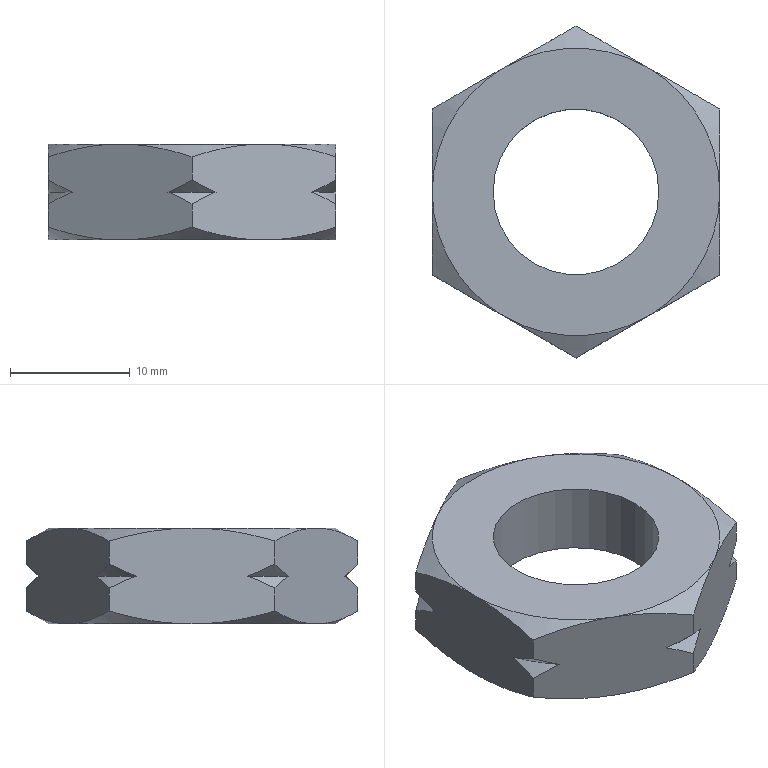Part | STEP file | HXGR200008-06-03-04_M16 | 1 solid | 39 faces | box 24 x 27.713 x 8 mm | volume 2454 mm3 | cone 26 | plane 9 | cylinder 4 | commonest cylinder face diameters 13.835 x2 19.5 x2
STEP:
#1=CARTESIAN_POINT('',(9.75,0.,2.));
#2=VERTEX_POINT('',#1);
#3=CARTESIAN_POINT('',(-9.75,0.,2.));
#4=VERTEX_POINT('',#3);
#5=CARTESIAN_POINT('',(0.,0.,2.));
#6=DIRECTION('',(0.,0.,-1.));
#7=DIRECTION('',(-1.,0.,0.));
#8=AXIS2_PLACEMENT_3D('',#5,#6,#7);
#9=CIRCLE('',#8,9.75);
#10=EDGE_CURVE('',#2,#4,#9,.T.);
#11=ORIENTED_EDGE('',*,*,#10,.F.);
#12=CARTESIAN_POINT('',(9.75,0.,0.));
#13=VERTEX_POINT('',#12);
#14=CARTESIAN_POINT('',(9.75,0.,2.));
#15=DIRECTION('',(0.,0.,-1.));
#16=VECTOR('',#15,1000.);
#17=LINE('',#14,#16);
#18=EDGE_CURVE('',#2,#13,#17,.T.);
#19=ORIENTED_EDGE('',*,*,#18,.T.);
#20=CARTESIAN_POINT('',(-9.75,0.,0.));
#21=VERTEX_POINT('',#20);
#22=CARTESIAN_POINT('',(0.,0.,0.));
#23=DIRECTION('',(0.,0.,-1.));
#24=DIRECTION('',(-1.,0.,0.));
#25=AXIS2_PLACEMENT_3D('',#22,#23,#24);
#26=CIRCLE('',#25,9.75);
#27=EDGE_CURVE('',#13,#21,#26,.T.);
#28=ORIENTED_EDGE('',*,*,#27,.T.);
#29=CARTESIAN_POINT('',(-9.75,0.,2.));
#30=DIRECTION('',(0.,0.,-1.));
#31=VECTOR('',#30,1000.);
#32=LINE('',#29,#31);
#33=EDGE_CURVE('',#4,#21,#32,.T.);
#34=ORIENTED_EDGE('',*,*,#33,.F.);
#35=EDGE_LOOP('',(#11,#19,#28,#34));
#36=FACE_OUTER_BOUND('',#35,.T.);
#37=CARTESIAN_POINT('',(0.,0.,2.));
#38=DIRECTION('',(0.,0.,-1.));
#39=DIRECTION('',(-1.,0.,0.));
#40=AXIS2_PLACEMENT_3D('',#37,#38,#39);
#41=CYLINDRICAL_SURFACE('',#40,9.75);
#42=ADVANCED_FACE('',(#36),#41,.F.);
#43=CARTESIAN_POINT('',(-6.918,0.,8.));
#44=VERTEX_POINT('',#43);
#45=CARTESIAN_POINT('',(6.918,0.,8.));
#46=VERTEX_POINT('',#45);
#47=CARTESIAN_POINT('',(0.,0.,8.));
#48=DIRECTION('',(0.,0.,1.));
#49=DIRECTION('',(1.,0.,0.));
#50=AXIS2_PLACEMENT_3D('',#47,#48,#49);
#51=CIRCLE('',#50,6.918);
#52=EDGE_CURVE('',#44,#46,#51,.T.);
#53=ORIENTED_EDGE('',*,*,#52,.T.);
#54=CARTESIAN_POINT('',(6.918,0.,2.));
#55=VERTEX_POINT('',#54);
#56=CARTESIAN_POINT('',(6.918,0.,8.));
#57=DIRECTION('',(0.,0.,-1.));
#58=VECTOR('',#57,1000.);
#59=LINE('',#56,#58);
#60=EDGE_CURVE('',#46,#55,#59,.T.);
#61=ORIENTED_EDGE('',*,*,#60,.T.);
#62=CARTESIAN_POINT('',(-6.918,0.,2.));
#63=VERTEX_POINT('',#62);
#64=CARTESIAN_POINT('',(0.,0.,2.));
#65=DIRECTION('',(0.,0.,-1.));
#66=DIRECTION('',(-1.,0.,0.));
#67=AXIS2_PLACEMENT_3D('',#64,#65,#66);
#68=CIRCLE('',#67,6.918);
#69=EDGE_CURVE('',#55,#63,#68,.T.);
#70=ORIENTED_EDGE('',*,*,#69,.T.);
#71=CARTESIAN_POINT('',(-6.918,0.,8.));
#72=DIRECTION('',(0.,0.,-1.));
#73=VECTOR('',#72,1000.);
#74=LINE('',#71,#73);
#75=EDGE_CURVE('',#44,#63,#74,.T.);
#76=ORIENTED_EDGE('',*,*,#75,.F.);
#77=EDGE_LOOP('',(#53,#61,#70,#76));
#78=FACE_OUTER_BOUND('',#77,.T.);
#79=CARTESIAN_POINT('',(0.,0.,8.));
#80=DIRECTION('',(0.,0.,-1.));
#81=DIRECTION('',(-1.,0.,0.));
#82=AXIS2_PLACEMENT_3D('',#79,#80,#81);
#83=CYLINDRICAL_SURFACE('',#82,6.918);
#84=ADVANCED_FACE('',(#78),#83,.F.);
#85=CARTESIAN_POINT('',(9.996,8.085,4.));
#86=VERTEX_POINT('',#85);
#87=CARTESIAN_POINT('',(12.,6.928,5.));
#88=VERTEX_POINT('',#87);
#89=CARTESIAN_POINT('',(9.996,8.085,4.));
#90=CARTESIAN_POINT('',(10.339,7.887,4.142));
#91=CARTESIAN_POINT('',(10.68,7.69,4.3));
#92=CARTESIAN_POINT('',(11.348,7.305,4.635));
#93=CARTESIAN_POINT('',(11.676,7.115,4.813));
#94=CARTESIAN_POINT('',(12.,6.928,5.));
#95=B_SPLINE_CURVE_WITH_KNOTS('',3,(#89,#90,#91,#92,#93,#94),.UNSPECIFIED.,.F.,.F.,(4,2,4),(0.02361,0.02487,0.02612),.UNSPECIFIED.);
#96=EDGE_CURVE('',#86,#88,#95,.T.);
#97=ORIENTED_EDGE('',*,*,#96,.F.);
#98=CARTESIAN_POINT('',(12.,6.928,3.));
#99=VERTEX_POINT('',#98);
#100=CARTESIAN_POINT('',(12.,6.928,3.));
#101=CARTESIAN_POINT('',(11.348,7.305,3.377));
#102=CARTESIAN_POINT('',(10.682,7.689,3.716));
#103=CARTESIAN_POINT('',(9.996,8.085,4.));
#104=B_SPLINE_CURVE_WITH_KNOTS('',3,(#100,#101,#102,#103),.UNSPECIFIED.,.F.,.F.,(4,4),(0.01167,0.01419),.UNSPECIFIED.);
#105=EDGE_CURVE('',#99,#86,#104,.T.);
#106=ORIENTED_EDGE('',*,*,#105,.F.);
#107=CARTESIAN_POINT('',(12.,6.928,1.072));
#108=VERTEX_POINT('',#107);
#109=CARTESIAN_POINT('',(12.,6.928,8.));
#110=DIRECTION('',(0.,0.,-1.));
#111=VECTOR('',#110,1000.);
#112=LINE('',#109,#111);
#113=EDGE_CURVE('',#99,#108,#112,.T.);
#114=ORIENTED_EDGE('',*,*,#113,.T.);
#115=CARTESIAN_POINT('',(6.,10.392,0.));
#116=VERTEX_POINT('',#115);
#117=CARTESIAN_POINT('',(6.,10.392,0.));
#118=CARTESIAN_POINT('',(6.509,10.098,0.));
#119=CARTESIAN_POINT('',(7.021,9.803,0.02533));
#120=CARTESIAN_POINT('',(8.033,9.219,0.1234));
#121=CARTESIAN_POINT('',(8.535,8.929,0.196));
#122=CARTESIAN_POINT('',(10.034,8.063,0.476));
#123=CARTESIAN_POINT('',(11.021,7.493,0.7454));
#124=CARTESIAN_POINT('',(12.,6.928,1.072));
#125=B_SPLINE_CURVE_WITH_KNOTS('',3,(#117,#118,#119,#120,#121,#122,#123,#124),.UNSPECIFIED.,.F.,.F.,(4,2,2,4),(0.00701,0.008756,0.0105,0.01399),.UNSPECIFIED.);
#126=EDGE_CURVE('',#116,#108,#125,.T.);
#127=ORIENTED_EDGE('',*,*,#126,.F.);
#128=CARTESIAN_POINT('',(0.,13.856,1.072));
#129=VERTEX_POINT('',#128);
#130=CARTESIAN_POINT('',(0.,13.856,1.072));
#131=CARTESIAN_POINT('',(0.9815,13.29,0.7446));
#132=CARTESIAN_POINT('',(1.97,12.719,0.4751));
#133=CARTESIAN_POINT('',(3.968,11.565,0.1021));
#134=CARTESIAN_POINT('',(4.978,10.982,0.));
#135=CARTESIAN_POINT('',(6.,10.392,0.));
#136=B_SPLINE_CURVE_WITH_KNOTS('',3,(#130,#131,#132,#133,#134,#135),.UNSPECIFIED.,.F.,.F.,(4,2,4),(0.000000238,0.003505,0.00701),.UNSPECIFIED.);
#137=EDGE_CURVE('',#129,#116,#136,.T.);
#138=ORIENTED_EDGE('',*,*,#137,.F.);
#139=CARTESIAN_POINT('',(0.,13.856,3.));
#140=VERTEX_POINT('',#139);
#141=CARTESIAN_POINT('',(0.,13.856,8.));
#142=DIRECTION('',(0.,0.,-1.));
#143=VECTOR('',#142,1000.);
#144=LINE('',#141,#143);
#145=EDGE_CURVE('',#140,#129,#144,.T.);
#146=ORIENTED_EDGE('',*,*,#145,.F.);
#147=CARTESIAN_POINT('',(2.004,12.699,4.));
#148=VERTEX_POINT('',#147);
#149=CARTESIAN_POINT('',(2.004,12.699,4.));
#150=CARTESIAN_POINT('',(1.661,12.898,3.858));
#151=CARTESIAN_POINT('',(1.32,13.094,3.7));
#152=CARTESIAN_POINT('',(0.6518,13.48,3.365));
#153=CARTESIAN_POINT('',(0.3236,13.67,3.187));
#154=CARTESIAN_POINT('',(0.,13.856,3.));
#155=B_SPLINE_CURVE_WITH_KNOTS('',3,(#149,#150,#151,#152,#153,#154),.UNSPECIFIED.,.F.,.F.,(4,2,4),(0.02361,0.02487,0.02612),.UNSPECIFIED.);
#156=EDGE_CURVE('',#148,#140,#155,.T.);
#157=ORIENTED_EDGE('',*,*,#156,.F.);
#158=CARTESIAN_POINT('',(0.,13.856,5.));
#159=VERTEX_POINT('',#158);
#160=CARTESIAN_POINT('',(0.,13.856,5.));
#161=CARTESIAN_POINT('',(0.6523,13.48,4.623));
#162=CARTESIAN_POINT('',(1.318,13.095,4.284));
#163=CARTESIAN_POINT('',(2.004,12.699,4.));
#164=B_SPLINE_CURVE_WITH_KNOTS('',3,(#160,#161,#162,#163),.UNSPECIFIED.,.F.,.F.,(4,4),(0.01167,0.01419),.UNSPECIFIED.);
#165=EDGE_CURVE('',#159,#148,#164,.T.);
#166=ORIENTED_EDGE('',*,*,#165,.F.);
#167=CARTESIAN_POINT('',(0.,13.856,6.928));
#168=VERTEX_POINT('',#167);
#169=CARTESIAN_POINT('',(0.,13.856,8.));
#170=DIRECTION('',(0.,0.,-1.));
#171=VECTOR('',#170,1000.);
#172=LINE('',#169,#171);
#173=EDGE_CURVE('',#168,#159,#172,.T.);
#174=ORIENTED_EDGE('',*,*,#173,.F.);
#175=CARTESIAN_POINT('',(6.,10.392,8.));
#176=VERTEX_POINT('',#175);
#177=CARTESIAN_POINT('',(6.,10.392,8.));
#178=CARTESIAN_POINT('',(5.491,10.686,8.));
#179=CARTESIAN_POINT('',(4.979,10.982,7.975));
#180=CARTESIAN_POINT('',(3.967,11.566,7.877));
#181=CARTESIAN_POINT('',(3.465,11.856,7.804));
#182=CARTESIAN_POINT('',(1.966,12.721,7.524));
#183=CARTESIAN_POINT('',(0.9791,13.291,7.255));
#184=CARTESIAN_POINT('',(0.,13.856,6.928));
#185=B_SPLINE_CURVE_WITH_KNOTS('',3,(#177,#178,#179,#180,#181,#182,#183,#184),.UNSPECIFIED.,.F.,.F.,(4,2,2,4),(0.00701,0.008756,0.0105,0.01399),.UNSPECIFIED.);
#186=EDGE_CURVE('',#176,#168,#185,.T.);
#187=ORIENTED_EDGE('',*,*,#186,.F.);
#188=CARTESIAN_POINT('',(12.,6.928,6.928));
#189=VERTEX_POINT('',#188);
#190=CARTESIAN_POINT('',(12.,6.928,6.928));
#191=CARTESIAN_POINT('',(11.018,7.495,7.255));
#192=CARTESIAN_POINT('',(10.03,8.066,7.525));
#193=CARTESIAN_POINT('',(8.032,9.219,7.898));
#194=CARTESIAN_POINT('',(7.022,9.802,8.));
#195=CARTESIAN_POINT('',(6.,10.392,8.));
#196=B_SPLINE_CURVE_WITH_KNOTS('',3,(#190,#191,#192,#193,#194,#195),.UNSPECIFIED.,.F.,.F.,(4,2,4),(0.000000238,0.003505,0.00701),.UNSPECIFIED.);
#197=EDGE_CURVE('',#189,#176,#196,.T.);
#198=ORIENTED_EDGE('',*,*,#197,.F.);
#199=CARTESIAN_POINT('',(12.,6.928,8.));
#200=DIRECTION('',(0.,0.,-1.));
#201=VECTOR('',#200,1000.);
#202=LINE('',#199,#201);
#203=EDGE_CURVE('',#189,#88,#202,.T.);
#204=ORIENTED_EDGE('',*,*,#203,.T.);
#205=EDGE_LOOP('',(#97,#106,#114,#127,#138,#146,#157,#166,#174,#187,#198,#204));
#206=FACE_OUTER_BOUND('',#205,.T.);
#207=CARTESIAN_POINT('',(12.,6.928,8.));
#208=DIRECTION('',(-0.5,-0.866,0.));
#209=DIRECTION('',(0.866,-0.5,0.));
#210=AXIS2_PLACEMENT_3D('',#207,#208,#209);
#211=PLANE('',#210);
#212=ADVANCED_FACE('',(#206),#211,.F.);
#213=CARTESIAN_POINT('',(-2.004,12.699,4.));
#214=VERTEX_POINT('',#213);
#215=CARTESIAN_POINT('',(-2.004,12.699,4.));
#216=CARTESIAN_POINT('',(-1.661,12.898,4.142));
#217=CARTESIAN_POINT('',(-1.32,13.094,4.3));
#218=CARTESIAN_POINT('',(-0.6518,13.48,4.635));
#219=CARTESIAN_POINT('',(-0.3236,13.67,4.813));
#220=CARTESIAN_POINT('',(0.,13.856,5.));
#221=B_SPLINE_CURVE_WITH_KNOTS('',3,(#215,#216,#217,#218,#219,#220),.UNSPECIFIED.,.F.,.F.,(4,2,4),(0.02361,0.02487,0.02612),.UNSPECIFIED.);
#222=EDGE_CURVE('',#214,#159,#221,.T.);
#223=ORIENTED_EDGE('',*,*,#222,.F.);
#224=CARTESIAN_POINT('',(0.,13.856,3.));
#225=CARTESIAN_POINT('',(-0.6523,13.48,3.377));
#226=CARTESIAN_POINT('',(-1.318,13.095,3.716));
#227=CARTESIAN_POINT('',(-2.004,12.699,4.));
#228=B_SPLINE_CURVE_WITH_KNOTS('',3,(#224,#225,#226,#227),.UNSPECIFIED.,.F.,.F.,(4,4),(0.01167,0.01419),.UNSPECIFIED.);
#229=EDGE_CURVE('',#140,#214,#228,.T.);
#230=ORIENTED_EDGE('',*,*,#229,.F.);
#231=ORIENTED_EDGE('',*,*,#145,.T.);
#232=CARTESIAN_POINT('',(-6.,10.392,0.));
#233=VERTEX_POINT('',#232);
#234=CARTESIAN_POINT('',(-6.,10.392,0.));
#235=CARTESIAN_POINT('',(-5.491,10.686,0.));
#236=CARTESIAN_POINT('',(-4.979,10.982,0.02533));
#237=CARTESIAN_POINT('',(-3.967,11.566,0.1234));
#238=CARTESIAN_POINT('',(-3.465,11.856,0.196));
#239=CARTESIAN_POINT('',(-1.966,12.721,0.476));
#240=CARTESIAN_POINT('',(-0.9791,13.291,0.7454));
#241=CARTESIAN_POINT('',(0.,13.856,1.072));
#242=B_SPLINE_CURVE_WITH_KNOTS('',3,(#234,#235,#236,#237,#238,#239,#240,#241),.UNSPECIFIED.,.F.,.F.,(4,2,2,4),(0.00701,0.008756,0.0105,0.01399),.UNSPECIFIED.);
#243=EDGE_CURVE('',#233,#129,#242,.T.);
#244=ORIENTED_EDGE('',*,*,#243,.F.);
#245=CARTESIAN_POINT('',(-12.,6.928,1.072));
#246=VERTEX_POINT('',#245);
#247=CARTESIAN_POINT('',(-12.,6.928,1.072));
#248=CARTESIAN_POINT('',(-11.018,7.495,0.7446));
#249=CARTESIAN_POINT('',(-10.03,8.066,0.4751));
#250=CARTESIAN_POINT('',(-8.032,9.219,0.1021));
#251=CARTESIAN_POINT('',(-7.022,9.802,0.));
#252=CARTESIAN_POINT('',(-6.,10.392,0.));
#253=B_SPLINE_CURVE_WITH_KNOTS('',3,(#247,#248,#249,#250,#251,#252),.UNSPECIFIED.,.F.,.F.,(4,2,4),(0.000000238,0.003505,0.00701),.UNSPECIFIED.);
#254=EDGE_CURVE('',#246,#233,#253,.T.);
#255=ORIENTED_EDGE('',*,*,#254,.F.);
#256=CARTESIAN_POINT('',(-12.,6.928,3.));
#257=VERTEX_POINT('',#256);
#258=CARTESIAN_POINT('',(-12.,6.928,8.));
#259=DIRECTION('',(0.,0.,-1.));
#260=VECTOR('',#259,1000.);
#261=LINE('',#258,#260);
#262=EDGE_CURVE('',#257,#246,#261,.T.);
#263=ORIENTED_EDGE('',*,*,#262,.F.);
#264=CARTESIAN_POINT('',(-9.996,8.085,4.));
#265=VERTEX_POINT('',#264);
#266=CARTESIAN_POINT('',(-9.996,8.085,4.));
#267=CARTESIAN_POINT('',(-10.339,7.887,3.858));
#268=CARTESIAN_POINT('',(-10.68,7.69,3.7));
#269=CARTESIAN_POINT('',(-11.348,7.305,3.365));
#270=CARTESIAN_POINT('',(-11.676,7.115,3.187));
#271=CARTESIAN_POINT('',(-12.,6.928,3.));
#272=B_SPLINE_CURVE_WITH_KNOTS('',3,(#266,#267,#268,#269,#270,#271),.UNSPECIFIED.,.F.,.F.,(4,2,4),(0.02361,0.02487,0.02612),.UNSPECIFIED.);
#273=EDGE_CURVE('',#265,#257,#272,.T.);
#274=ORIENTED_EDGE('',*,*,#273,.F.);
#275=CARTESIAN_POINT('',(-12.,6.928,5.));
#276=VERTEX_POINT('',#275);
#277=CARTESIAN_POINT('',(-12.,6.928,5.));
#278=CARTESIAN_POINT('',(-11.348,7.305,4.623));
#279=CARTESIAN_POINT('',(-10.682,7.689,4.284));
#280=CARTESIAN_POINT('',(-9.996,8.085,4.));
#281=B_SPLINE_CURVE_WITH_KNOTS('',3,(#277,#278,#279,#280),.UNSPECIFIED.,.F.,.F.,(4,4),(0.01167,0.01419),.UNSPECIFIED.);
#282=EDGE_CURVE('',#276,#265,#281,.T.);
#283=ORIENTED_EDGE('',*,*,#282,.F.);
#284=CARTESIAN_POINT('',(-12.,6.928,6.928));
#285=VERTEX_POINT('',#284);
#286=CARTESIAN_POINT('',(-12.,6.928,8.));
#287=DIRECTION('',(0.,0.,-1.));
#288=VECTOR('',#287,1000.);
#289=LINE('',#286,#288);
#290=EDGE_CURVE('',#285,#276,#289,.T.);
#291=ORIENTED_EDGE('',*,*,#290,.F.);
#292=CARTESIAN_POINT('',(-6.,10.392,8.));
#293=VERTEX_POINT('',#292);
#294=CARTESIAN_POINT('',(-6.,10.392,8.));
#295=CARTESIAN_POINT('',(-6.509,10.098,8.));
#296=CARTESIAN_POINT('',(-7.021,9.803,7.975));
#297=CARTESIAN_POINT('',(-8.033,9.219,7.877));
#298=CARTESIAN_POINT('',(-8.535,8.929,7.804));
#299=CARTESIAN_POINT('',(-10.034,8.063,7.524));
#300=CARTESIAN_POINT('',(-11.021,7.493,7.255));
#301=CARTESIAN_POINT('',(-12.,6.928,6.928));
#302=B_SPLINE_CURVE_WITH_KNOTS('',3,(#294,#295,#296,#297,#298,#299,#300,#301),.UNSPECIFIED.,.F.,.F.,(4,2,2,4),(0.00701,0.008756,0.0105,0.01399),.UNSPECIFIED.);
#303=EDGE_CURVE('',#293,#285,#302,.T.);
#304=ORIENTED_EDGE('',*,*,#303,.F.);
#305=CARTESIAN_POINT('',(0.,13.856,6.928));
#306=CARTESIAN_POINT('',(-0.9815,13.29,7.255));
#307=CARTESIAN_POINT('',(-1.97,12.719,7.525));
#308=CARTESIAN_POINT('',(-3.968,11.565,7.898));
#309=CARTESIAN_POINT('',(-4.978,10.982,8.));
#310=CARTESIAN_POINT('',(-6.,10.392,8.));
#311=B_SPLINE_CURVE_WITH_KNOTS('',3,(#305,#306,#307,#308,#309,#310),.UNSPECIFIED.,.F.,.F.,(4,2,4),(0.000000238,0.003505,0.00701),.UNSPECIFIED.);
#312=EDGE_CURVE('',#168,#293,#311,.T.);
#313=ORIENTED_EDGE('',*,*,#312,.F.);
#314=ORIENTED_EDGE('',*,*,#173,.T.);
#315=EDGE_LOOP('',(#223,#230,#231,#244,#255,#263,#274,#283,#291,#304,#313,#314));
#316=FACE_OUTER_BOUND('',#315,.T.);
#317=CARTESIAN_POINT('',(0.,13.856,8.));
#318=DIRECTION('',(0.5,-0.866,0.));
#319=DIRECTION('',(0.866,0.5,0.));
#320=AXIS2_PLACEMENT_3D('',#317,#318,#319);
#321=PLANE('',#320);
#322=ADVANCED_FACE('',(#316),#321,.F.);
#323=CARTESIAN_POINT('',(-12.,4.614,4.));
#324=VERTEX_POINT('',#323);
#325=CARTESIAN_POINT('',(-12.,4.614,4.));
#326=CARTESIAN_POINT('',(-12.,5.408,4.285));
#327=CARTESIAN_POINT('',(-12.,6.176,4.624));
#328=CARTESIAN_POINT('',(-12.,6.928,5.));
#329=B_SPLINE_CURVE_WITH_KNOTS('',3,(#325,#326,#327,#328),.UNSPECIFIED.,.F.,.F.,(4,4),(0.02193,0.02445),.UNSPECIFIED.);
#330=EDGE_CURVE('',#324,#276,#329,.T.);
#331=ORIENTED_EDGE('',*,*,#330,.F.);
#332=CARTESIAN_POINT('',(-12.,6.928,3.));
#333=CARTESIAN_POINT('',(-12.,6.552,3.188));
#334=CARTESIAN_POINT('',(-12.,6.17,3.368));
#335=CARTESIAN_POINT('',(-12.,5.398,3.703));
#336=CARTESIAN_POINT('',(-12.,5.008,3.859));
#337=CARTESIAN_POINT('',(-12.,4.614,4.));
#338=B_SPLINE_CURVE_WITH_KNOTS('',3,(#332,#333,#334,#335,#336,#337),.UNSPECIFIED.,.F.,.F.,(4,2,4),(0.01002,0.01127,0.01252),.UNSPECIFIED.);
#339=EDGE_CURVE('',#257,#324,#338,.T.);
#340=ORIENTED_EDGE('',*,*,#339,.F.);
#341=ORIENTED_EDGE('',*,*,#262,.T.);
#342=CARTESIAN_POINT('',(-12.,0.,0.));
#343=VERTEX_POINT('',#342);
#344=CARTESIAN_POINT('',(-12.,0.,0.));
#345=CARTESIAN_POINT('',(-12.,0.5865,0.));
#346=CARTESIAN_POINT('',(-12.,1.176,0.02506));
#347=CARTESIAN_POINT('',(-12.,2.355,0.1242));
#348=CARTESIAN_POINT('',(-12.,2.939,0.1976));
#349=CARTESIAN_POINT('',(-12.,4.673,0.4791));
#350=CARTESIAN_POINT('',(-12.,5.808,0.7483));
#351=CARTESIAN_POINT('',(-12.,6.928,1.072));
#352=B_SPLINE_CURVE_WITH_KNOTS('',3,(#344,#345,#346,#347,#348,#349,#350,#351),.UNSPECIFIED.,.F.,.F.,(4,2,2,4),(0.01983,0.02158,0.02334,0.02685),.UNSPECIFIED.);
#353=EDGE_CURVE('',#343,#246,#352,.T.);
#354=ORIENTED_EDGE('',*,*,#353,.F.);
#355=CARTESIAN_POINT('',(-12.,-6.928,1.072));
#356=VERTEX_POINT('',#355);
#357=CARTESIAN_POINT('',(-12.,-6.928,1.072));
#358=CARTESIAN_POINT('',(-12.,-5.8,0.7461));
#359=CARTESIAN_POINT('',(-12.,-4.647,0.4736));
#360=CARTESIAN_POINT('',(-12.,-2.335,0.1008));
#361=CARTESIAN_POINT('',(-12.,-1.172,0.));
#362=CARTESIAN_POINT('',(-12.,0.,0.));
#363=B_SPLINE_CURVE_WITH_KNOTS('',3,(#357,#358,#359,#360,#361,#362),.UNSPECIFIED.,.F.,.F.,(4,2,4),(0.01282,0.01632,0.01983),.UNSPECIFIED.);
#364=EDGE_CURVE('',#356,#343,#363,.T.);
#365=ORIENTED_EDGE('',*,*,#364,.F.);
#366=CARTESIAN_POINT('',(-12.,-6.928,3.));
#367=VERTEX_POINT('',#366);
#368=CARTESIAN_POINT('',(-12.,-6.928,8.));
#369=DIRECTION('',(0.,0.,-1.));
#370=VECTOR('',#369,1000.);
#371=LINE('',#368,#370);
#372=EDGE_CURVE('',#367,#356,#371,.T.);
#373=ORIENTED_EDGE('',*,*,#372,.F.);
#374=CARTESIAN_POINT('',(-12.,-4.614,4.));
#375=VERTEX_POINT('',#374);
#376=CARTESIAN_POINT('',(-12.,-4.614,4.));
#377=CARTESIAN_POINT('',(-12.,-5.408,3.715));
#378=CARTESIAN_POINT('',(-12.,-6.176,3.376));
#379=CARTESIAN_POINT('',(-12.,-6.928,3.));
#380=B_SPLINE_CURVE_WITH_KNOTS('',3,(#376,#377,#378,#379),.UNSPECIFIED.,.F.,.F.,(4,4),(0.02193,0.02445),.UNSPECIFIED.);
#381=EDGE_CURVE('',#375,#367,#380,.T.);
#382=ORIENTED_EDGE('',*,*,#381,.F.);
#383=CARTESIAN_POINT('',(-12.,-6.928,5.));
#384=VERTEX_POINT('',#383);
#385=CARTESIAN_POINT('',(-12.,-6.928,5.));
#386=CARTESIAN_POINT('',(-12.,-6.552,4.812));
#387=CARTESIAN_POINT('',(-12.,-6.17,4.632));
#388=CARTESIAN_POINT('',(-12.,-5.398,4.297));
#389=CARTESIAN_POINT('',(-12.,-5.008,4.141));
#390=CARTESIAN_POINT('',(-12.,-4.614,4.));
#391=B_SPLINE_CURVE_WITH_KNOTS('',3,(#385,#386,#387,#388,#389,#390),.UNSPECIFIED.,.F.,.F.,(4,2,4),(0.01002,0.01127,0.01252),.UNSPECIFIED.);
#392=EDGE_CURVE('',#384,#375,#391,.T.);
#393=ORIENTED_EDGE('',*,*,#392,.F.);
#394=CARTESIAN_POINT('',(-12.,-6.928,6.928));
#395=VERTEX_POINT('',#394);
#396=CARTESIAN_POINT('',(-12.,-6.928,8.));
#397=DIRECTION('',(0.,0.,-1.));
#398=VECTOR('',#397,1000.);
#399=LINE('',#396,#398);
#400=EDGE_CURVE('',#395,#384,#399,.T.);
#401=ORIENTED_EDGE('',*,*,#400,.F.);
#402=CARTESIAN_POINT('',(-12.,0.,8.));
#403=VERTEX_POINT('',#402);
#404=CARTESIAN_POINT('',(-12.,0.,8.));
#405=CARTESIAN_POINT('',(-12.,-1.172,8.));
#406=CARTESIAN_POINT('',(-12.,-2.335,7.899));
#407=CARTESIAN_POINT('',(-12.,-4.647,7.526));
#408=CARTESIAN_POINT('',(-12.,-5.8,7.254));
#409=CARTESIAN_POINT('',(-12.,-6.928,6.928));
#410=B_SPLINE_CURVE_WITH_KNOTS('',3,(#404,#405,#406,#407,#408,#409),.UNSPECIFIED.,.F.,.F.,(4,2,4),(0.04318,0.04669,0.05019),.UNSPECIFIED.);
#411=EDGE_CURVE('',#403,#395,#410,.T.);
#412=ORIENTED_EDGE('',*,*,#411,.F.);
#413=CARTESIAN_POINT('',(-12.,6.928,6.928));
#414=CARTESIAN_POINT('',(-12.,5.808,7.252));
#415=CARTESIAN_POINT('',(-12.,4.673,7.521));
#416=CARTESIAN_POINT('',(-12.,2.939,7.802));
#417=CARTESIAN_POINT('',(-12.,2.355,7.876));
#418=CARTESIAN_POINT('',(-12.,1.176,7.975));
#419=CARTESIAN_POINT('',(-12.,0.5865,8.));
#420=CARTESIAN_POINT('',(-12.,0.,8.));
#421=B_SPLINE_CURVE_WITH_KNOTS('',3,(#413,#414,#415,#416,#417,#418,#419,#420),.UNSPECIFIED.,.F.,.F.,(4,2,2,4),(0.03616,0.03967,0.04143,0.04318),.UNSPECIFIED.);
#422=EDGE_CURVE('',#285,#403,#421,.T.);
#423=ORIENTED_EDGE('',*,*,#422,.F.);
#424=ORIENTED_EDGE('',*,*,#290,.T.);
#425=EDGE_LOOP('',(#331,#340,#341,#354,#365,#373,#382,#393,#401,#412,#423,#424));
#426=FACE_OUTER_BOUND('',#425,.T.);
#427=CARTESIAN_POINT('',(-12.,6.928,8.));
#428=DIRECTION('',(1.,0.,0.));
#429=DIRECTION('',(0.,1.,0.));
#430=AXIS2_PLACEMENT_3D('',#427,#428,#429);
#431=PLANE('',#430);
#432=ADVANCED_FACE('',(#426),#431,.F.);
#433=CARTESIAN_POINT('',(-9.996,-8.085,4.));
#434=VERTEX_POINT('',#433);
#435=CARTESIAN_POINT('',(-9.996,-8.085,4.));
#436=CARTESIAN_POINT('',(-10.339,-7.887,4.142));
#437=CARTESIAN_POINT('',(-10.68,-7.69,4.3));
#438=CARTESIAN_POINT('',(-11.348,-7.305,4.635));
#439=CARTESIAN_POINT('',(-11.676,-7.115,4.813));
#440=CARTESIAN_POINT('',(-12.,-6.928,5.));
#441=B_SPLINE_CURVE_WITH_KNOTS('',3,(#435,#436,#437,#438,#439,#440),.UNSPECIFIED.,.F.,.F.,(4,2,4),(0.02361,0.02487,0.02612),.UNSPECIFIED.);
#442=EDGE_CURVE('',#434,#384,#441,.T.);
#443=ORIENTED_EDGE('',*,*,#442,.F.);
#444=CARTESIAN_POINT('',(-12.,-6.928,3.));
#445=CARTESIAN_POINT('',(-11.348,-7.305,3.377));
#446=CARTESIAN_POINT('',(-10.682,-7.689,3.716));
#447=CARTESIAN_POINT('',(-9.996,-8.085,4.));
#448=B_SPLINE_CURVE_WITH_KNOTS('',3,(#444,#445,#446,#447),.UNSPECIFIED.,.F.,.F.,(4,4),(0.01167,0.01419),.UNSPECIFIED.);
#449=EDGE_CURVE('',#367,#434,#448,.T.);
#450=ORIENTED_EDGE('',*,*,#449,.F.);
#451=ORIENTED_EDGE('',*,*,#372,.T.);
#452=CARTESIAN_POINT('',(-6.,-10.392,0.));
#453=VERTEX_POINT('',#452);
#454=CARTESIAN_POINT('',(-6.,-10.392,0.));
#455=CARTESIAN_POINT('',(-6.509,-10.098,0.));
#456=CARTESIAN_POINT('',(-7.021,-9.803,0.02533));
#457=CARTESIAN_POINT('',(-8.033,-9.219,0.1234));
#458=CARTESIAN_POINT('',(-8.535,-8.929,0.196));
#459=CARTESIAN_POINT('',(-10.034,-8.063,0.476));
#460=CARTESIAN_POINT('',(-11.021,-7.493,0.7454));
#461=CARTESIAN_POINT('',(-12.,-6.928,1.072));
#462=B_SPLINE_CURVE_WITH_KNOTS('',3,(#454,#455,#456,#457,#458,#459,#460,#461),.UNSPECIFIED.,.F.,.F.,(4,2,2,4),(0.00701,0.008756,0.0105,0.01399),.UNSPECIFIED.);
#463=EDGE_CURVE('',#453,#356,#462,.T.);
#464=ORIENTED_EDGE('',*,*,#463,.F.);
#465=CARTESIAN_POINT('',(0.,-13.856,1.072));
#466=VERTEX_POINT('',#465);
#467=CARTESIAN_POINT('',(0.,-13.856,1.072));
#468=CARTESIAN_POINT('',(-0.9815,-13.29,0.7446));
#469=CARTESIAN_POINT('',(-1.97,-12.719,0.4751));
#470=CARTESIAN_POINT('',(-3.968,-11.565,0.1021));
#471=CARTESIAN_POINT('',(-4.978,-10.982,0.));
#472=CARTESIAN_POINT('',(-6.,-10.392,0.));
#473=B_SPLINE_CURVE_WITH_KNOTS('',3,(#467,#468,#469,#470,#471,#472),.UNSPECIFIED.,.F.,.F.,(4,2,4),(0.000000238,0.003505,0.00701),.UNSPECIFIED.);
#474=EDGE_CURVE('',#466,#453,#473,.T.);
#475=ORIENTED_EDGE('',*,*,#474,.F.);
#476=CARTESIAN_POINT('',(0.,-13.856,3.));
#477=VERTEX_POINT('',#476);
#478=CARTESIAN_POINT('',(0.,-13.856,8.));
#479=DIRECTION('',(0.,0.,-1.));
#480=VECTOR('',#479,1000.);
#481=LINE('',#478,#480);
#482=EDGE_CURVE('',#477,#466,#481,.T.);
#483=ORIENTED_EDGE('',*,*,#482,.F.);
#484=CARTESIAN_POINT('',(-2.004,-12.699,4.));
#485=VERTEX_POINT('',#484);
#486=CARTESIAN_POINT('',(-2.004,-12.699,4.));
#487=CARTESIAN_POINT('',(-1.661,-12.898,3.858));
#488=CARTESIAN_POINT('',(-1.32,-13.094,3.7));
#489=CARTESIAN_POINT('',(-0.6518,-13.48,3.365));
#490=CARTESIAN_POINT('',(-0.3236,-13.67,3.187));
#491=CARTESIAN_POINT('',(0.,-13.856,3.));
#492=B_SPLINE_CURVE_WITH_KNOTS('',3,(#486,#487,#488,#489,#490,#491),.UNSPECIFIED.,.F.,.F.,(4,2,4),(0.02361,0.02487,0.02612),.UNSPECIFIED.);
#493=EDGE_CURVE('',#485,#477,#492,.T.);
#494=ORIENTED_EDGE('',*,*,#493,.F.);
#495=CARTESIAN_POINT('',(0.,-13.856,5.));
#496=VERTEX_POINT('',#495);
#497=CARTESIAN_POINT('',(0.,-13.856,5.));
#498=CARTESIAN_POINT('',(-0.6523,-13.48,4.623));
#499=CARTESIAN_POINT('',(-1.318,-13.095,4.284));
#500=CARTESIAN_POINT('',(-2.004,-12.699,4.));
#501=B_SPLINE_CURVE_WITH_KNOTS('',3,(#497,#498,#499,#500),.UNSPECIFIED.,.F.,.F.,(4,4),(0.01167,0.01419),.UNSPECIFIED.);
#502=EDGE_CURVE('',#496,#485,#501,.T.);
#503=ORIENTED_EDGE('',*,*,#502,.F.);
#504=CARTESIAN_POINT('',(0.,-13.856,6.928));
#505=VERTEX_POINT('',#504);
#506=CARTESIAN_POINT('',(0.,-13.856,8.));
#507=DIRECTION('',(0.,0.,-1.));
#508=VECTOR('',#507,1000.);
#509=LINE('',#506,#508);
#510=EDGE_CURVE('',#505,#496,#509,.T.);
#511=ORIENTED_EDGE('',*,*,#510,.F.);
#512=CARTESIAN_POINT('',(-6.,-10.392,8.));
#513=VERTEX_POINT('',#512);
#514=CARTESIAN_POINT('',(-6.,-10.392,8.));
#515=CARTESIAN_POINT('',(-5.491,-10.686,8.));
#516=CARTESIAN_POINT('',(-4.979,-10.982,7.975));
#517=CARTESIAN_POINT('',(-3.967,-11.566,7.877));
#518=CARTESIAN_POINT('',(-3.465,-11.856,7.804));
#519=CARTESIAN_POINT('',(-1.966,-12.721,7.524));
#520=CARTESIAN_POINT('',(-0.9791,-13.291,7.255));
#521=CARTESIAN_POINT('',(0.,-13.856,6.928));
#522=B_SPLINE_CURVE_WITH_KNOTS('',3,(#514,#515,#516,#517,#518,#519,#520,#521),.UNSPECIFIED.,.F.,.F.,(4,2,2,4),(0.00701,0.008756,0.0105,0.01399),.UNSPECIFIED.);
#523=EDGE_CURVE('',#513,#505,#522,.T.);
#524=ORIENTED_EDGE('',*,*,#523,.F.);
#525=CARTESIAN_POINT('',(-12.,-6.928,6.928));
#526=CARTESIAN_POINT('',(-11.018,-7.495,7.255));
#527=CARTESIAN_POINT('',(-10.03,-8.066,7.525));
#528=CARTESIAN_POINT('',(-8.032,-9.219,7.898));
#529=CARTESIAN_POINT('',(-7.022,-9.802,8.));
#530=CARTESIAN_POINT('',(-6.,-10.392,8.));
#531=B_SPLINE_CURVE_WITH_KNOTS('',3,(#525,#526,#527,#528,#529,#530),.UNSPECIFIED.,.F.,.F.,(4,2,4),(0.000000238,0.003505,0.00701),.UNSPECIFIED.);
#532=EDGE_CURVE('',#395,#513,#531,.T.);
#533=ORIENTED_EDGE('',*,*,#532,.F.);
#534=ORIENTED_EDGE('',*,*,#400,.T.);
#535=EDGE_LOOP('',(#443,#450,#451,#464,#475,#483,#494,#503,#511,#524,#533,#534));
#536=FACE_OUTER_BOUND('',#535,.T.);
#537=CARTESIAN_POINT('',(-12.,-6.928,8.));
#538=DIRECTION('',(0.5,0.866,0.));
#539=DIRECTION('',(-0.866,0.5,0.));
#540=AXIS2_PLACEMENT_3D('',#537,#538,#539);
#541=PLANE('',#540);
#542=ADVANCED_FACE('',(#536),#541,.F.);
#543=CARTESIAN_POINT('',(2.004,-12.699,4.));
#544=VERTEX_POINT('',#543);
#545=CARTESIAN_POINT('',(2.004,-12.699,4.));
#546=CARTESIAN_POINT('',(1.661,-12.898,4.142));
#547=CARTESIAN_POINT('',(1.32,-13.094,4.3));
#548=CARTESIAN_POINT('',(0.6518,-13.48,4.635));
#549=CARTESIAN_POINT('',(0.3236,-13.67,4.813));
#550=CARTESIAN_POINT('',(0.,-13.856,5.));
#551=B_SPLINE_CURVE_WITH_KNOTS('',3,(#545,#546,#547,#548,#549,#550),.UNSPECIFIED.,.F.,.F.,(4,2,4),(0.02361,0.02487,0.02612),.UNSPECIFIED.);
#552=EDGE_CURVE('',#544,#496,#551,.T.);
#553=ORIENTED_EDGE('',*,*,#552,.F.);
#554=CARTESIAN_POINT('',(0.,-13.856,3.));
#555=CARTESIAN_POINT('',(0.6523,-13.48,3.377));
#556=CARTESIAN_POINT('',(1.318,-13.095,3.716));
#557=CARTESIAN_POINT('',(2.004,-12.699,4.));
#558=B_SPLINE_CURVE_WITH_KNOTS('',3,(#554,#555,#556,#557),.UNSPECIFIED.,.F.,.F.,(4,4),(0.01167,0.01419),.UNSPECIFIED.);
#559=EDGE_CURVE('',#477,#544,#558,.T.);
#560=ORIENTED_EDGE('',*,*,#559,.F.);
#561=ORIENTED_EDGE('',*,*,#482,.T.);
#562=CARTESIAN_POINT('',(6.,-10.392,0.));
#563=VERTEX_POINT('',#562);
#564=CARTESIAN_POINT('',(6.,-10.392,0.));
#565=CARTESIAN_POINT('',(5.491,-10.686,0.));
#566=CARTESIAN_POINT('',(4.979,-10.982,0.02533));
#567=CARTESIAN_POINT('',(3.967,-11.566,0.1234));
#568=CARTESIAN_POINT('',(3.465,-11.856,0.196));
#569=CARTESIAN_POINT('',(1.966,-12.721,0.476));
#570=CARTESIAN_POINT('',(0.9791,-13.291,0.7454));
#571=CARTESIAN_POINT('',(0.,-13.856,1.072));
#572=B_SPLINE_CURVE_WITH_KNOTS('',3,(#564,#565,#566,#567,#568,#569,#570,#571),.UNSPECIFIED.,.F.,.F.,(4,2,2,4),(0.00701,0.008756,0.0105,0.01399),.UNSPECIFIED.);
#573=EDGE_CURVE('',#563,#466,#572,.T.);
#574=ORIENTED_EDGE('',*,*,#573,.F.);
#575=CARTESIAN_POINT('',(12.,-6.928,1.072));
#576=VERTEX_POINT('',#575);
#577=CARTESIAN_POINT('',(12.,-6.928,1.072));
#578=CARTESIAN_POINT('',(11.018,-7.495,0.7446));
#579=CARTESIAN_POINT('',(10.03,-8.066,0.4751));
#580=CARTESIAN_POINT('',(8.032,-9.219,0.1021));
#581=CARTESIAN_POINT('',(7.022,-9.802,0.));
#582=CARTESIAN_POINT('',(6.,-10.392,0.));
#583=B_SPLINE_CURVE_WITH_KNOTS('',3,(#577,#578,#579,#580,#581,#582),.UNSPECIFIED.,.F.,.F.,(4,2,4),(0.000000238,0.003505,0.00701),.UNSPECIFIED.);
#584=EDGE_CURVE('',#576,#563,#583,.T.);
#585=ORIENTED_EDGE('',*,*,#584,.F.);
#586=CARTESIAN_POINT('',(12.,-6.928,3.));
#587=VERTEX_POINT('',#586);
#588=CARTESIAN_POINT('',(12.,-6.928,8.));
#589=DIRECTION('',(0.,0.,-1.));
#590=VECTOR('',#589,1000.);
#591=LINE('',#588,#590);
#592=EDGE_CURVE('',#587,#576,#591,.T.);
#593=ORIENTED_EDGE('',*,*,#592,.F.);
#594=CARTESIAN_POINT('',(9.996,-8.085,4.));
#595=VERTEX_POINT('',#594);
#596=CARTESIAN_POINT('',(9.996,-8.085,4.));
#597=CARTESIAN_POINT('',(10.339,-7.887,3.858));
#598=CARTESIAN_POINT('',(10.68,-7.69,3.7));
#599=CARTESIAN_POINT('',(11.348,-7.305,3.365));
#600=CARTESIAN_POINT('',(11.676,-7.115,3.187));
#601=CARTESIAN_POINT('',(12.,-6.928,3.));
#602=B_SPLINE_CURVE_WITH_KNOTS('',3,(#596,#597,#598,#599,#600,#601),.UNSPECIFIED.,.F.,.F.,(4,2,4),(0.02361,0.02487,0.02612),.UNSPECIFIED.);
#603=EDGE_CURVE('',#595,#587,#602,.T.);
#604=ORIENTED_EDGE('',*,*,#603,.F.);
#605=CARTESIAN_POINT('',(12.,-6.928,5.));
#606=VERTEX_POINT('',#605);
#607=CARTESIAN_POINT('',(12.,-6.928,5.));
#608=CARTESIAN_POINT('',(11.348,-7.305,4.623));
#609=CARTESIAN_POINT('',(10.682,-7.689,4.284));
#610=CARTESIAN_POINT('',(9.996,-8.085,4.));
#611=B_SPLINE_CURVE_WITH_KNOTS('',3,(#607,#608,#609,#610),.UNSPECIFIED.,.F.,.F.,(4,4),(0.01167,0.01419),.UNSPECIFIED.);
#612=EDGE_CURVE('',#606,#595,#611,.T.);
#613=ORIENTED_EDGE('',*,*,#612,.F.);
#614=CARTESIAN_POINT('',(12.,-6.928,6.928));
#615=VERTEX_POINT('',#614);
#616=CARTESIAN_POINT('',(12.,-6.928,8.));
#617=DIRECTION('',(0.,0.,-1.));
#618=VECTOR('',#617,1000.);
#619=LINE('',#616,#618);
#620=EDGE_CURVE('',#615,#606,#619,.T.);
#621=ORIENTED_EDGE('',*,*,#620,.F.);
#622=CARTESIAN_POINT('',(6.,-10.392,8.));
#623=VERTEX_POINT('',#622);
#624=CARTESIAN_POINT('',(6.,-10.392,8.));
#625=CARTESIAN_POINT('',(6.509,-10.098,8.));
#626=CARTESIAN_POINT('',(7.021,-9.803,7.975));
#627=CARTESIAN_POINT('',(8.033,-9.219,7.877));
#628=CARTESIAN_POINT('',(8.535,-8.929,7.804));
#629=CARTESIAN_POINT('',(10.034,-8.063,7.524));
#630=CARTESIAN_POINT('',(11.021,-7.493,7.255));
#631=CARTESIAN_POINT('',(12.,-6.928,6.928));
#632=B_SPLINE_CURVE_WITH_KNOTS('',3,(#624,#625,#626,#627,#628,#629,#630,#631),.UNSPECIFIED.,.F.,.F.,(4,2,2,4),(0.00701,0.008756,0.0105,0.01399),.UNSPECIFIED.);
#633=EDGE_CURVE('',#623,#615,#632,.T.);
#634=ORIENTED_EDGE('',*,*,#633,.F.);
#635=CARTESIAN_POINT('',(0.,-13.856,6.928));
#636=CARTESIAN_POINT('',(0.9815,-13.29,7.255));
#637=CARTESIAN_POINT('',(1.97,-12.719,7.525));
#638=CARTESIAN_POINT('',(3.968,-11.565,7.898));
#639=CARTESIAN_POINT('',(4.978,-10.982,8.));
#640=CARTESIAN_POINT('',(6.,-10.392,8.));
#641=B_SPLINE_CURVE_WITH_KNOTS('',3,(#635,#636,#637,#638,#639,#640),.UNSPECIFIED.,.F.,.F.,(4,2,4),(0.000000238,0.003505,0.00701),.UNSPECIFIED.);
#642=EDGE_CURVE('',#505,#623,#641,.T.);
#643=ORIENTED_EDGE('',*,*,#642,.F.);
#644=ORIENTED_EDGE('',*,*,#510,.T.);
#645=EDGE_LOOP('',(#553,#560,#561,#574,#585,#593,#604,#613,#621,#634,#643,#644));
#646=FACE_OUTER_BOUND('',#645,.T.);
#647=CARTESIAN_POINT('',(0.,-13.856,8.));
#648=DIRECTION('',(-0.5,0.866,0.));
#649=DIRECTION('',(-0.866,-0.5,0.));
#650=AXIS2_PLACEMENT_3D('',#647,#648,#649);
#651=PLANE('',#650);
#652=ADVANCED_FACE('',(#646),#651,.F.);
#653=CARTESIAN_POINT('',(12.,-4.614,4.));
#654=VERTEX_POINT('',#653);
#655=CARTESIAN_POINT('',(12.,-4.614,4.));
#656=CARTESIAN_POINT('',(12.,-5.408,4.285));
#657=CARTESIAN_POINT('',(12.,-6.176,4.624));
#658=CARTESIAN_POINT('',(12.,-6.928,5.));
#659=B_SPLINE_CURVE_WITH_KNOTS('',3,(#655,#656,#657,#658),.UNSPECIFIED.,.F.,.F.,(4,4),(0.02193,0.02445),.UNSPECIFIED.);
#660=EDGE_CURVE('',#654,#606,#659,.T.);
#661=ORIENTED_EDGE('',*,*,#660,.F.);
#662=CARTESIAN_POINT('',(12.,-6.928,3.));
#663=CARTESIAN_POINT('',(12.,-6.552,3.188));
#664=CARTESIAN_POINT('',(12.,-6.17,3.368));
#665=CARTESIAN_POINT('',(12.,-5.398,3.703));
#666=CARTESIAN_POINT('',(12.,-5.008,3.859));
#667=CARTESIAN_POINT('',(12.,-4.614,4.));
#668=B_SPLINE_CURVE_WITH_KNOTS('',3,(#662,#663,#664,#665,#666,#667),.UNSPECIFIED.,.F.,.F.,(4,2,4),(0.01002,0.01127,0.01252),.UNSPECIFIED.);
#669=EDGE_CURVE('',#587,#654,#668,.T.);
#670=ORIENTED_EDGE('',*,*,#669,.F.);
#671=ORIENTED_EDGE('',*,*,#592,.T.);
#672=CARTESIAN_POINT('',(12.,0.,0.));
#673=VERTEX_POINT('',#672);
#674=CARTESIAN_POINT('',(12.,0.,0.));
#675=CARTESIAN_POINT('',(12.,-1.172,0.));
#676=CARTESIAN_POINT('',(12.,-2.335,0.1008));
#677=CARTESIAN_POINT('',(12.,-4.647,0.4736));
#678=CARTESIAN_POINT('',(12.,-5.8,0.7461));
#679=CARTESIAN_POINT('',(12.,-6.928,1.072));
#680=B_SPLINE_CURVE_WITH_KNOTS('',3,(#674,#675,#676,#677,#678,#679),.UNSPECIFIED.,.F.,.F.,(4,2,4),(0.04318,0.04669,0.05019),.UNSPECIFIED.);
#681=EDGE_CURVE('',#673,#576,#680,.T.);
#682=ORIENTED_EDGE('',*,*,#681,.F.);
#683=CARTESIAN_POINT('',(12.,6.928,1.072));
#684=CARTESIAN_POINT('',(12.,5.808,0.7483));
#685=CARTESIAN_POINT('',(12.,4.673,0.4791));
#686=CARTESIAN_POINT('',(12.,2.939,0.1976));
#687=CARTESIAN_POINT('',(12.,2.355,0.1242));
#688=CARTESIAN_POINT('',(12.,1.176,0.02506));
#689=CARTESIAN_POINT('',(12.,0.5865,0.));
#690=CARTESIAN_POINT('',(12.,0.,0.));
#691=B_SPLINE_CURVE_WITH_KNOTS('',3,(#683,#684,#685,#686,#687,#688,#689,#690),.UNSPECIFIED.,.F.,.F.,(4,2,2,4),(0.03616,0.03967,0.04143,0.04318),.UNSPECIFIED.);
#692=EDGE_CURVE('',#108,#673,#691,.T.);
#693=ORIENTED_EDGE('',*,*,#692,.F.);
#694=ORIENTED_EDGE('',*,*,#113,.F.);
#695=CARTESIAN_POINT('',(12.,4.614,4.));
#696=VERTEX_POINT('',#695);
#697=CARTESIAN_POINT('',(12.,4.614,4.));
#698=CARTESIAN_POINT('',(12.,5.408,3.715));
#699=CARTESIAN_POINT('',(12.,6.176,3.376));
#700=CARTESIAN_POINT('',(12.,6.928,3.));
#701=B_SPLINE_CURVE_WITH_KNOTS('',3,(#697,#698,#699,#700),.UNSPECIFIED.,.F.,.F.,(4,4),(0.02193,0.02445),.UNSPECIFIED.);
#702=EDGE_CURVE('',#696,#99,#701,.T.);
#703=ORIENTED_EDGE('',*,*,#702,.F.);
#704=CARTESIAN_POINT('',(12.,6.928,5.));
#705=CARTESIAN_POINT('',(12.,6.552,4.812));
#706=CARTESIAN_POINT('',(12.,6.17,4.632));
#707=CARTESIAN_POINT('',(12.,5.398,4.297));
#708=CARTESIAN_POINT('',(12.,5.008,4.141));
#709=CARTESIAN_POINT('',(12.,4.614,4.));
#710=B_SPLINE_CURVE_WITH_KNOTS('',3,(#704,#705,#706,#707,#708,#709),.UNSPECIFIED.,.F.,.F.,(4,2,4),(0.01002,0.01127,0.01252),.UNSPECIFIED.);
#711=EDGE_CURVE('',#88,#696,#710,.T.);
#712=ORIENTED_EDGE('',*,*,#711,.F.);
#713=ORIENTED_EDGE('',*,*,#203,.F.);
#714=CARTESIAN_POINT('',(12.,0.,8.));
#715=VERTEX_POINT('',#714);
#716=CARTESIAN_POINT('',(12.,0.,8.));
#717=CARTESIAN_POINT('',(12.,0.5865,8.));
#718=CARTESIAN_POINT('',(12.,1.176,7.975));
#719=CARTESIAN_POINT('',(12.,2.355,7.876));
#720=CARTESIAN_POINT('',(12.,2.939,7.802));
#721=CARTESIAN_POINT('',(12.,4.673,7.521));
#722=CARTESIAN_POINT('',(12.,5.808,7.252));
#723=CARTESIAN_POINT('',(12.,6.928,6.928));
#724=B_SPLINE_CURVE_WITH_KNOTS('',3,(#716,#717,#718,#719,#720,#721,#722,#723),.UNSPECIFIED.,.F.,.F.,(4,2,2,4),(0.01983,0.02158,0.02334,0.02685),.UNSPECIFIED.);
#725=EDGE_CURVE('',#715,#189,#724,.T.);
#726=ORIENTED_EDGE('',*,*,#725,.F.);
#727=CARTESIAN_POINT('',(12.,-6.928,6.928));
#728=CARTESIAN_POINT('',(12.,-5.8,7.254));
#729=CARTESIAN_POINT('',(12.,-4.647,7.526));
#730=CARTESIAN_POINT('',(12.,-2.335,7.899));
#731=CARTESIAN_POINT('',(12.,-1.172,8.));
#732=CARTESIAN_POINT('',(12.,0.,8.));
#733=B_SPLINE_CURVE_WITH_KNOTS('',3,(#727,#728,#729,#730,#731,#732),.UNSPECIFIED.,.F.,.F.,(4,2,4),(0.01282,0.01632,0.01983),.UNSPECIFIED.);
#734=EDGE_CURVE('',#615,#715,#733,.T.);
#735=ORIENTED_EDGE('',*,*,#734,.F.);
#736=ORIENTED_EDGE('',*,*,#620,.T.);
#737=EDGE_LOOP('',(#661,#670,#671,#682,#693,#694,#703,#712,#713,#726,#735,#736));
#738=FACE_OUTER_BOUND('',#737,.T.);
#739=CARTESIAN_POINT('',(12.,-6.928,8.));
#740=DIRECTION('',(-1.,0.,0.));
#741=DIRECTION('',(0.,-1.,0.));
#742=AXIS2_PLACEMENT_3D('',#739,#740,#741);
#743=PLANE('',#742);
#744=ADVANCED_FACE('',(#738),#743,.F.);
#745=ORIENTED_EDGE('',*,*,#60,.F.);
#746=CARTESIAN_POINT('',(0.,0.,8.));
#747=DIRECTION('',(0.,0.,1.));
#748=DIRECTION('',(1.,0.,0.));
#749=AXIS2_PLACEMENT_3D('',#746,#747,#748);
#750=CIRCLE('',#749,6.918);
#751=EDGE_CURVE('',#46,#44,#750,.T.);
#752=ORIENTED_EDGE('',*,*,#751,.T.);
#753=ORIENTED_EDGE('',*,*,#75,.T.);
#754=CARTESIAN_POINT('',(0.,0.,2.));
#755=DIRECTION('',(0.,0.,-1.));
#756=DIRECTION('',(-1.,0.,0.));
#757=AXIS2_PLACEMENT_3D('',#754,#755,#756);
#758=CIRCLE('',#757,6.918);
#759=EDGE_CURVE('',#63,#55,#758,.T.);
#760=ORIENTED_EDGE('',*,*,#759,.T.);
#761=EDGE_LOOP('',(#745,#752,#753,#760));
#762=FACE_OUTER_BOUND('',#761,.T.);
#763=CARTESIAN_POINT('',(0.,0.,8.));
#764=DIRECTION('',(0.,0.,-1.));
#765=DIRECTION('',(-1.,0.,0.));
#766=AXIS2_PLACEMENT_3D('',#763,#764,#765);
#767=CYLINDRICAL_SURFACE('',#766,6.918);
#768=ADVANCED_FACE('',(#762),#767,.F.);
#769=ORIENTED_EDGE('',*,*,#52,.F.);
#770=ORIENTED_EDGE('',*,*,#751,.F.);
#771=EDGE_LOOP('',(#769,#770));
#772=FACE_BOUND('',#771,.T.);
#773=CARTESIAN_POINT('',(0.,0.,8.));
#774=DIRECTION('',(0.,0.,-1.));
#775=DIRECTION('',(-1.,0.,0.));
#776=AXIS2_PLACEMENT_3D('',#773,#774,#775);
#777=CIRCLE('',#776,12.);
#778=EDGE_CURVE('',#403,#293,#777,.T.);
#779=ORIENTED_EDGE('',*,*,#778,.F.);
#780=CARTESIAN_POINT('',(0.,0.,8.));
#781=DIRECTION('',(0.,0.,-1.));
#782=DIRECTION('',(-1.,0.,0.));
#783=AXIS2_PLACEMENT_3D('',#780,#781,#782);
#784=CIRCLE('',#783,12.);
#785=EDGE_CURVE('',#513,#403,#784,.T.);
#786=ORIENTED_EDGE('',*,*,#785,.F.);
#787=CARTESIAN_POINT('',(0.,0.,8.));
#788=DIRECTION('',(0.,0.,-1.));
#789=DIRECTION('',(-1.,0.,0.));
#790=AXIS2_PLACEMENT_3D('',#787,#788,#789);
#791=CIRCLE('',#790,12.);
#792=EDGE_CURVE('',#623,#513,#791,.T.);
#793=ORIENTED_EDGE('',*,*,#792,.F.);
#794=CARTESIAN_POINT('',(0.,0.,8.));
#795=DIRECTION('',(0.,0.,-1.));
#796=DIRECTION('',(-1.,0.,0.));
#797=AXIS2_PLACEMENT_3D('',#794,#795,#796);
#798=CIRCLE('',#797,12.);
#799=EDGE_CURVE('',#715,#623,#798,.T.);
#800=ORIENTED_EDGE('',*,*,#799,.F.);
#801=CARTESIAN_POINT('',(0.,0.,8.));
#802=DIRECTION('',(0.,0.,1.));
#803=DIRECTION('',(1.,0.,0.));
#804=AXIS2_PLACEMENT_3D('',#801,#802,#803);
#805=CIRCLE('',#804,12.);
#806=EDGE_CURVE('',#715,#176,#805,.T.);
#807=ORIENTED_EDGE('',*,*,#806,.T.);
#808=CARTESIAN_POINT('',(0.,0.,8.));
#809=DIRECTION('',(0.,0.,-1.));
#810=DIRECTION('',(-1.,0.,0.));
#811=AXIS2_PLACEMENT_3D('',#808,#809,#810);
#812=CIRCLE('',#811,12.);
#813=EDGE_CURVE('',#293,#176,#812,.T.);
#814=ORIENTED_EDGE('',*,*,#813,.F.);
#815=EDGE_LOOP('',(#779,#786,#793,#800,#807,#814));
#816=FACE_OUTER_BOUND('',#815,.T.);
#817=CARTESIAN_POINT('',(12.,6.928,8.));
#818=DIRECTION('',(0.,0.,-1.));
#819=DIRECTION('',(-1.,0.,0.));
#820=AXIS2_PLACEMENT_3D('',#817,#818,#819);
#821=PLANE('',#820);
#822=ADVANCED_FACE('',(#772,#816),#821,.F.);
#823=CARTESIAN_POINT('',(0.,0.,0.));
#824=DIRECTION('',(0.,0.,-1.));
#825=DIRECTION('',(-1.,0.,0.));
#826=AXIS2_PLACEMENT_3D('',#823,#824,#825);
#827=CIRCLE('',#826,9.75);
#828=EDGE_CURVE('',#21,#13,#827,.T.);
#829=ORIENTED_EDGE('',*,*,#828,.F.);
#830=ORIENTED_EDGE('',*,*,#27,.F.);
#831=EDGE_LOOP('',(#829,#830));
#832=FACE_BOUND('',#831,.T.);
#833=CARTESIAN_POINT('',(0.,0.,0.));
#834=DIRECTION('',(0.,0.,-1.));
#835=DIRECTION('',(-1.,0.,0.));
#836=AXIS2_PLACEMENT_3D('',#833,#834,#835);
#837=CIRCLE('',#836,12.);
#838=EDGE_CURVE('',#453,#343,#837,.T.);
#839=ORIENTED_EDGE('',*,*,#838,.T.);
#840=CARTESIAN_POINT('',(0.,0.,0.));
#841=DIRECTION('',(0.,0.,-1.));
#842=DIRECTION('',(-1.,0.,0.));
#843=AXIS2_PLACEMENT_3D('',#840,#841,#842);
#844=CIRCLE('',#843,12.);
#845=EDGE_CURVE('',#343,#233,#844,.T.);
#846=ORIENTED_EDGE('',*,*,#845,.T.);
#847=CARTESIAN_POINT('',(0.,0.,0.));
#848=DIRECTION('',(0.,0.,-1.));
#849=DIRECTION('',(-1.,0.,0.));
#850=AXIS2_PLACEMENT_3D('',#847,#848,#849);
#851=CIRCLE('',#850,12.);
#852=EDGE_CURVE('',#233,#116,#851,.T.);
#853=ORIENTED_EDGE('',*,*,#852,.T.);
#854=CARTESIAN_POINT('',(0.,0.,0.));
#855=DIRECTION('',(0.,0.,-1.));
#856=DIRECTION('',(-1.,0.,0.));
#857=AXIS2_PLACEMENT_3D('',#854,#855,#856);
#858=CIRCLE('',#857,12.);
#859=EDGE_CURVE('',#116,#673,#858,.T.);
#860=ORIENTED_EDGE('',*,*,#859,.T.);
#861=CARTESIAN_POINT('',(0.,0.,0.));
#862=DIRECTION('',(0.,0.,-1.));
#863=DIRECTION('',(-1.,0.,0.));
#864=AXIS2_PLACEMENT_3D('',#861,#862,#863);
#865=CIRCLE('',#864,12.);
#866=EDGE_CURVE('',#673,#563,#865,.T.);
#867=ORIENTED_EDGE('',*,*,#866,.T.);
#868=CARTESIAN_POINT('',(0.,0.,0.));
#869=DIRECTION('',(0.,0.,-1.));
#870=DIRECTION('',(-1.,0.,0.));
#871=AXIS2_PLACEMENT_3D('',#868,#869,#870);
#872=CIRCLE('',#871,12.);
#873=EDGE_CURVE('',#563,#453,#872,.T.);
#874=ORIENTED_EDGE('',*,*,#873,.T.);
#875=EDGE_LOOP('',(#839,#846,#853,#860,#867,#874));
#876=FACE_OUTER_BOUND('',#875,.T.);
#877=CARTESIAN_POINT('',(12.,6.928,0.));
#878=DIRECTION('',(0.,0.,-1.));
#879=DIRECTION('',(-1.,0.,0.));
#880=AXIS2_PLACEMENT_3D('',#877,#878,#879);
#881=PLANE('',#880);
#882=ADVANCED_FACE('',(#832,#876),#881,.T.);
#883=ORIENTED_EDGE('',*,*,#584,.T.);
#884=ORIENTED_EDGE('',*,*,#866,.F.);
#885=ORIENTED_EDGE('',*,*,#681,.T.);
#886=EDGE_LOOP('',(#883,#884,#885));
#887=FACE_OUTER_BOUND('',#886,.T.);
#888=CARTESIAN_POINT('',(0.,0.,0.));
#889=DIRECTION('',(0.,0.,1.));
#890=DIRECTION('',(-1.,0.,0.));
#891=AXIS2_PLACEMENT_3D('',#888,#889,#890);
#892=CONICAL_SURFACE('',#891,12.,1.047);
#893=ADVANCED_FACE('',(#887),#892,.T.);
#894=ORIENTED_EDGE('',*,*,#126,.T.);
#895=ORIENTED_EDGE('',*,*,#692,.T.);
#896=ORIENTED_EDGE('',*,*,#859,.F.);
#897=EDGE_LOOP('',(#894,#895,#896));
#898=FACE_OUTER_BOUND('',#897,.T.);
#899=CARTESIAN_POINT('',(0.,0.,0.));
#900=DIRECTION('',(0.,0.,1.));
#901=DIRECTION('',(-1.,0.,0.));
#902=AXIS2_PLACEMENT_3D('',#899,#900,#901);
#903=CONICAL_SURFACE('',#902,12.,1.047);
#904=ADVANCED_FACE('',(#898),#903,.T.);
#905=ORIENTED_EDGE('',*,*,#474,.T.);
#906=ORIENTED_EDGE('',*,*,#873,.F.);
#907=ORIENTED_EDGE('',*,*,#573,.T.);
#908=EDGE_LOOP('',(#905,#906,#907));
#909=FACE_OUTER_BOUND('',#908,.T.);
#910=CARTESIAN_POINT('',(0.,0.,0.));
#911=DIRECTION('',(0.,0.,1.));
#912=DIRECTION('',(-1.,0.,0.));
#913=AXIS2_PLACEMENT_3D('',#910,#911,#912);
#914=CONICAL_SURFACE('',#913,12.,1.047);
#915=ADVANCED_FACE('',(#909),#914,.T.);
#916=ORIENTED_EDGE('',*,*,#364,.T.);
#917=ORIENTED_EDGE('',*,*,#838,.F.);
#918=ORIENTED_EDGE('',*,*,#463,.T.);
#919=EDGE_LOOP('',(#916,#917,#918));
#920=FACE_OUTER_BOUND('',#919,.T.);
#921=CARTESIAN_POINT('',(0.,0.,0.));
#922=DIRECTION('',(0.,0.,1.));
#923=DIRECTION('',(-1.,0.,0.));
#924=AXIS2_PLACEMENT_3D('',#921,#922,#923);
#925=CONICAL_SURFACE('',#924,12.,1.047);
#926=ADVANCED_FACE('',(#920),#925,.T.);
#927=ORIENTED_EDGE('',*,*,#353,.T.);
#928=ORIENTED_EDGE('',*,*,#254,.T.);
#929=ORIENTED_EDGE('',*,*,#845,.F.);
#930=EDGE_LOOP('',(#927,#928,#929));
#931=FACE_OUTER_BOUND('',#930,.T.);
#932=CARTESIAN_POINT('',(0.,0.,0.));
#933=DIRECTION('',(0.,0.,1.));
#934=DIRECTION('',(-1.,0.,0.));
#935=AXIS2_PLACEMENT_3D('',#932,#933,#934);
#936=CONICAL_SURFACE('',#935,12.,1.047);
#937=ADVANCED_FACE('',(#931),#936,.T.);
#938=ORIENTED_EDGE('',*,*,#243,.T.);
#939=ORIENTED_EDGE('',*,*,#137,.T.);
#940=ORIENTED_EDGE('',*,*,#852,.F.);
#941=EDGE_LOOP('',(#938,#939,#940));
#942=FACE_OUTER_BOUND('',#941,.T.);
#943=CARTESIAN_POINT('',(0.,0.,0.));
#944=DIRECTION('',(0.,0.,1.));
#945=DIRECTION('',(-1.,0.,0.));
#946=AXIS2_PLACEMENT_3D('',#943,#944,#945);
#947=CONICAL_SURFACE('',#946,12.,1.047);
#948=ADVANCED_FACE('',(#942),#947,.T.);
#949=ORIENTED_EDGE('',*,*,#411,.T.);
#950=ORIENTED_EDGE('',*,*,#532,.T.);
#951=ORIENTED_EDGE('',*,*,#785,.T.);
#952=EDGE_LOOP('',(#949,#950,#951));
#953=FACE_OUTER_BOUND('',#952,.T.);
#954=CARTESIAN_POINT('',(0.,0.,8.));
#955=DIRECTION('',(0.,0.,-1.));
#956=DIRECTION('',(1.,0.,0.));
#957=AXIS2_PLACEMENT_3D('',#954,#955,#956);
#958=CONICAL_SURFACE('',#957,12.,1.047);
#959=ADVANCED_FACE('',(#953),#958,.T.);
#960=ORIENTED_EDGE('',*,*,#523,.T.);
#961=ORIENTED_EDGE('',*,*,#642,.T.);
#962=ORIENTED_EDGE('',*,*,#792,.T.);
#963=EDGE_LOOP('',(#960,#961,#962));
#964=FACE_OUTER_BOUND('',#963,.T.);
#965=CARTESIAN_POINT('',(0.,0.,8.));
#966=DIRECTION('',(0.,0.,-1.));
#967=DIRECTION('',(1.,0.,0.));
#968=AXIS2_PLACEMENT_3D('',#965,#966,#967);
#969=CONICAL_SURFACE('',#968,12.,1.047);
#970=ADVANCED_FACE('',(#964),#969,.T.);
#971=ORIENTED_EDGE('',*,*,#633,.T.);
#972=ORIENTED_EDGE('',*,*,#734,.T.);
#973=ORIENTED_EDGE('',*,*,#799,.T.);
#974=EDGE_LOOP('',(#971,#972,#973));
#975=FACE_OUTER_BOUND('',#974,.T.);
#976=CARTESIAN_POINT('',(0.,0.,8.));
#977=DIRECTION('',(0.,0.,-1.));
#978=DIRECTION('',(1.,0.,0.));
#979=AXIS2_PLACEMENT_3D('',#976,#977,#978);
#980=CONICAL_SURFACE('',#979,12.,1.047);
#981=ADVANCED_FACE('',(#975),#980,.T.);
#982=ORIENTED_EDGE('',*,*,#197,.T.);
#983=ORIENTED_EDGE('',*,*,#806,.F.);
#984=ORIENTED_EDGE('',*,*,#725,.T.);
#985=EDGE_LOOP('',(#982,#983,#984));
#986=FACE_OUTER_BOUND('',#985,.T.);
#987=CARTESIAN_POINT('',(0.,0.,8.));
#988=DIRECTION('',(0.,0.,-1.));
#989=DIRECTION('',(1.,0.,0.));
#990=AXIS2_PLACEMENT_3D('',#987,#988,#989);
#991=CONICAL_SURFACE('',#990,12.,1.047);
#992=ADVANCED_FACE('',(#986),#991,.T.);
#993=ORIENTED_EDGE('',*,*,#186,.T.);
#994=ORIENTED_EDGE('',*,*,#312,.T.);
#995=ORIENTED_EDGE('',*,*,#813,.T.);
#996=EDGE_LOOP('',(#993,#994,#995));
#997=FACE_OUTER_BOUND('',#996,.T.);
#998=CARTESIAN_POINT('',(0.,0.,8.));
#999=DIRECTION('',(0.,0.,-1.));
#1000=DIRECTION('',(1.,0.,0.));
#1001=AXIS2_PLACEMENT_3D('',#998,#999,#1000);
#1002=CONICAL_SURFACE('',#1001,12.,1.047);
#1003=ADVANCED_FACE('',(#997),#1002,.T.);
#1004=ORIENTED_EDGE('',*,*,#303,.T.);
#1005=ORIENTED_EDGE('',*,*,#422,.T.);
#1006=ORIENTED_EDGE('',*,*,#778,.T.);
#1007=EDGE_LOOP('',(#1004,#1005,#1006));
#1008=FACE_OUTER_BOUND('',#1007,.T.);
#1009=CARTESIAN_POINT('',(0.,0.,8.));
#1010=DIRECTION('',(0.,0.,-1.));
#1011=DIRECTION('',(1.,0.,0.));
#1012=AXIS2_PLACEMENT_3D('',#1009,#1010,#1011);
#1013=CONICAL_SURFACE('',#1012,12.,1.047);
#1014=ADVANCED_FACE('',(#1008),#1013,.T.);
#1015=ORIENTED_EDGE('',*,*,#18,.F.);
#1016=CARTESIAN_POINT('',(0.,0.,2.));
#1017=DIRECTION('',(0.,0.,-1.));
#1018=DIRECTION('',(-1.,0.,0.));
#1019=AXIS2_PLACEMENT_3D('',#1016,#1017,#1018);
#1020=CIRCLE('',#1019,9.75);
#1021=EDGE_CURVE('',#4,#2,#1020,.T.);
#1022=ORIENTED_EDGE('',*,*,#1021,.F.);
#1023=ORIENTED_EDGE('',*,*,#33,.T.);
#1024=ORIENTED_EDGE('',*,*,#828,.T.);
#1025=EDGE_LOOP('',(#1015,#1022,#1023,#1024));
#1026=FACE_OUTER_BOUND('',#1025,.T.);
#1027=CARTESIAN_POINT('',(0.,0.,2.));
#1028=DIRECTION('',(0.,0.,-1.));
#1029=DIRECTION('',(-1.,0.,0.));
#1030=AXIS2_PLACEMENT_3D('',#1027,#1028,#1029);
#1031=CYLINDRICAL_SURFACE('',#1030,9.75);
#1032=ADVANCED_FACE('',(#1026),#1031,.F.);
#1033=ORIENTED_EDGE('',*,*,#759,.F.);
#1034=ORIENTED_EDGE('',*,*,#69,.F.);
#1035=EDGE_LOOP('',(#1033,#1034));
#1036=FACE_BOUND('',#1035,.T.);
#1037=ORIENTED_EDGE('',*,*,#1021,.T.);
#1038=ORIENTED_EDGE('',*,*,#10,.T.);
#1039=EDGE_LOOP('',(#1037,#1038));
#1040=FACE_OUTER_BOUND('',#1039,.T.);
#1041=CARTESIAN_POINT('',(0.,0.,2.));
#1042=DIRECTION('',(0.,0.,-1.));
#1043=DIRECTION('',(-1.,0.,0.));
#1044=AXIS2_PLACEMENT_3D('',#1041,#1042,#1043);
#1045=PLANE('',#1044);
#1046=ADVANCED_FACE('',(#1036,#1040),#1045,.T.);
#1047=ORIENTED_EDGE('',*,*,#105,.T.);
#1048=CARTESIAN_POINT('',(0.,0.,4.));
#1049=DIRECTION('',(0.,0.,1.));
#1050=DIRECTION('',(0.,1.,0.));
#1051=AXIS2_PLACEMENT_3D('',#1048,#1049,#1050);
#1052=CIRCLE('',#1051,12.856);
#1053=EDGE_CURVE('',#696,#86,#1052,.T.);
#1054=ORIENTED_EDGE('',*,*,#1053,.F.);
#1055=ORIENTED_EDGE('',*,*,#702,.T.);
#1056=EDGE_LOOP('',(#1047,#1054,#1055));
#1057=FACE_OUTER_BOUND('',#1056,.T.);
#1058=CARTESIAN_POINT('',(0.,0.,4.));
#1059=DIRECTION('',(0.,0.,-1.));
#1060=DIRECTION('',(-1.,0.,0.));
#1061=AXIS2_PLACEMENT_3D('',#1058,#1059,#1060);
#1062=CONICAL_SURFACE('',#1061,12.856,0.7854);
#1063=ADVANCED_FACE('',(#1057),#1062,.T.);
#1064=ORIENTED_EDGE('',*,*,#96,.T.);
#1065=ORIENTED_EDGE('',*,*,#711,.T.);
#1066=ORIENTED_EDGE('',*,*,#1053,.T.);
#1067=EDGE_LOOP('',(#1064,#1065,#1066));
#1068=FACE_OUTER_BOUND('',#1067,.T.);
#1069=CARTESIAN_POINT('',(0.,0.,5.));
#1070=DIRECTION('',(0.,0.,1.));
#1071=DIRECTION('',(1.,0.,0.));
#1072=AXIS2_PLACEMENT_3D('',#1069,#1070,#1071);
#1073=CONICAL_SURFACE('',#1072,13.856,0.7854);
#1074=ADVANCED_FACE('',(#1068),#1073,.T.);
#1075=ORIENTED_EDGE('',*,*,#603,.T.);
#1076=ORIENTED_EDGE('',*,*,#669,.T.);
#1077=CARTESIAN_POINT('',(0.,0.,4.));
#1078=DIRECTION('',(0.,0.,1.));
#1079=DIRECTION('',(0.,1.,0.));
#1080=AXIS2_PLACEMENT_3D('',#1077,#1078,#1079);
#1081=CIRCLE('',#1080,12.856);
#1082=EDGE_CURVE('',#595,#654,#1081,.T.);
#1083=ORIENTED_EDGE('',*,*,#1082,.F.);
#1084=EDGE_LOOP('',(#1075,#1076,#1083));
#1085=FACE_OUTER_BOUND('',#1084,.T.);
#1086=CARTESIAN_POINT('',(0.,0.,4.));
#1087=DIRECTION('',(0.,0.,-1.));
#1088=DIRECTION('',(-1.,0.,0.));
#1089=AXIS2_PLACEMENT_3D('',#1086,#1087,#1088);
#1090=CONICAL_SURFACE('',#1089,12.856,0.7854);
#1091=ADVANCED_FACE('',(#1085),#1090,.T.);
#1092=ORIENTED_EDGE('',*,*,#612,.T.);
#1093=ORIENTED_EDGE('',*,*,#1082,.T.);
#1094=ORIENTED_EDGE('',*,*,#660,.T.);
#1095=EDGE_LOOP('',(#1092,#1093,#1094));
#1096=FACE_OUTER_BOUND('',#1095,.T.);
#1097=CARTESIAN_POINT('',(0.,0.,5.));
#1098=DIRECTION('',(0.,0.,1.));
#1099=DIRECTION('',(1.,0.,0.));
#1100=AXIS2_PLACEMENT_3D('',#1097,#1098,#1099);
#1101=CONICAL_SURFACE('',#1100,13.856,0.7854);
#1102=ADVANCED_FACE('',(#1096),#1101,.T.);
#1103=ORIENTED_EDGE('',*,*,#493,.T.);
#1104=ORIENTED_EDGE('',*,*,#559,.T.);
#1105=CARTESIAN_POINT('',(0.,0.,4.));
#1106=DIRECTION('',(0.,0.,1.));
#1107=DIRECTION('',(0.,1.,0.));
#1108=AXIS2_PLACEMENT_3D('',#1105,#1106,#1107);
#1109=CIRCLE('',#1108,12.856);
#1110=EDGE_CURVE('',#485,#544,#1109,.T.);
#1111=ORIENTED_EDGE('',*,*,#1110,.F.);
#1112=EDGE_LOOP('',(#1103,#1104,#1111));
#1113=FACE_OUTER_BOUND('',#1112,.T.);
#1114=CARTESIAN_POINT('',(0.,0.,4.));
#1115=DIRECTION('',(0.,0.,-1.));
#1116=DIRECTION('',(-1.,0.,0.));
#1117=AXIS2_PLACEMENT_3D('',#1114,#1115,#1116);
#1118=CONICAL_SURFACE('',#1117,12.856,0.7854);
#1119=ADVANCED_FACE('',(#1113),#1118,.T.);
#1120=ORIENTED_EDGE('',*,*,#502,.T.);
#1121=ORIENTED_EDGE('',*,*,#1110,.T.);
#1122=ORIENTED_EDGE('',*,*,#552,.T.);
#1123=EDGE_LOOP('',(#1120,#1121,#1122));
#1124=FACE_OUTER_BOUND('',#1123,.T.);
#1125=CARTESIAN_POINT('',(0.,0.,5.));
#1126=DIRECTION('',(0.,0.,1.));
#1127=DIRECTION('',(1.,0.,0.));
#1128=AXIS2_PLACEMENT_3D('',#1125,#1126,#1127);
#1129=CONICAL_SURFACE('',#1128,13.856,0.7854);
#1130=ADVANCED_FACE('',(#1124),#1129,.T.);
#1131=ORIENTED_EDGE('',*,*,#381,.T.);
#1132=ORIENTED_EDGE('',*,*,#449,.T.);
#1133=CARTESIAN_POINT('',(0.,0.,4.));
#1134=DIRECTION('',(0.,0.,1.));
#1135=DIRECTION('',(0.,1.,0.));
#1136=AXIS2_PLACEMENT_3D('',#1133,#1134,#1135);
#1137=CIRCLE('',#1136,12.856);
#1138=EDGE_CURVE('',#375,#434,#1137,.T.);
#1139=ORIENTED_EDGE('',*,*,#1138,.F.);
#1140=EDGE_LOOP('',(#1131,#1132,#1139));
#1141=FACE_OUTER_BOUND('',#1140,.T.);
#1142=CARTESIAN_POINT('',(0.,0.,4.));
#1143=DIRECTION('',(0.,0.,-1.));
#1144=DIRECTION('',(-1.,0.,0.));
#1145=AXIS2_PLACEMENT_3D('',#1142,#1143,#1144);
#1146=CONICAL_SURFACE('',#1145,12.856,0.7854);
#1147=ADVANCED_FACE('',(#1141),#1146,.T.);
#1148=ORIENTED_EDGE('',*,*,#392,.T.);
#1149=ORIENTED_EDGE('',*,*,#1138,.T.);
#1150=ORIENTED_EDGE('',*,*,#442,.T.);
#1151=EDGE_LOOP('',(#1148,#1149,#1150));
#1152=FACE_OUTER_BOUND('',#1151,.T.);
#1153=CARTESIAN_POINT('',(0.,0.,5.));
#1154=DIRECTION('',(0.,0.,1.));
#1155=DIRECTION('',(1.,0.,0.));
#1156=AXIS2_PLACEMENT_3D('',#1153,#1154,#1155);
#1157=CONICAL_SURFACE('',#1156,13.856,0.7854);
#1158=ADVANCED_FACE('',(#1152),#1157,.T.);
#1159=ORIENTED_EDGE('',*,*,#273,.T.);
#1160=ORIENTED_EDGE('',*,*,#339,.T.);
#1161=CARTESIAN_POINT('',(0.,0.,4.));
#1162=DIRECTION('',(0.,0.,1.));
#1163=DIRECTION('',(0.,1.,0.));
#1164=AXIS2_PLACEMENT_3D('',#1161,#1162,#1163);
#1165=CIRCLE('',#1164,12.856);
#1166=EDGE_CURVE('',#265,#324,#1165,.T.);
#1167=ORIENTED_EDGE('',*,*,#1166,.F.);
#1168=EDGE_LOOP('',(#1159,#1160,#1167));
#1169=FACE_OUTER_BOUND('',#1168,.T.);
#1170=CARTESIAN_POINT('',(0.,0.,4.));
#1171=DIRECTION('',(0.,0.,-1.));
#1172=DIRECTION('',(-1.,0.,0.));
#1173=AXIS2_PLACEMENT_3D('',#1170,#1171,#1172);
#1174=CONICAL_SURFACE('',#1173,12.856,0.7854);
#1175=ADVANCED_FACE('',(#1169),#1174,.T.);
#1176=ORIENTED_EDGE('',*,*,#282,.T.);
#1177=ORIENTED_EDGE('',*,*,#1166,.T.);
#1178=ORIENTED_EDGE('',*,*,#330,.T.);
#1179=EDGE_LOOP('',(#1176,#1177,#1178));
#1180=FACE_OUTER_BOUND('',#1179,.T.);
#1181=CARTESIAN_POINT('',(0.,0.,5.));
#1182=DIRECTION('',(0.,0.,1.));
#1183=DIRECTION('',(1.,0.,0.));
#1184=AXIS2_PLACEMENT_3D('',#1181,#1182,#1183);
#1185=CONICAL_SURFACE('',#1184,13.856,0.7854);
#1186=ADVANCED_FACE('',(#1180),#1185,.T.);
#1187=ORIENTED_EDGE('',*,*,#165,.T.);
#1188=CARTESIAN_POINT('',(0.,12.856,4.));
#1189=VERTEX_POINT('',#1188);
#1190=CARTESIAN_POINT('',(0.,0.,4.));
#1191=DIRECTION('',(0.,0.,1.));
#1192=DIRECTION('',(0.,1.,0.));
#1193=AXIS2_PLACEMENT_3D('',#1190,#1191,#1192);
#1194=CIRCLE('',#1193,12.856);
#1195=EDGE_CURVE('',#148,#1189,#1194,.T.);
#1196=ORIENTED_EDGE('',*,*,#1195,.T.);
#1197=CARTESIAN_POINT('',(0.,13.856,5.));
#1198=DIRECTION('',(0.,-0.7071,-0.7071));
#1199=VECTOR('',#1198,1000.);
#1200=LINE('',#1197,#1199);
#1201=EDGE_CURVE('',#159,#1189,#1200,.T.);
#1202=ORIENTED_EDGE('',*,*,#1201,.F.);
#1203=EDGE_LOOP('',(#1187,#1196,#1202));
#1204=FACE_OUTER_BOUND('',#1203,.T.);
#1205=CARTESIAN_POINT('',(0.,0.,5.));
#1206=DIRECTION('',(0.,0.,1.));
#1207=DIRECTION('',(1.,0.,0.));
#1208=AXIS2_PLACEMENT_3D('',#1205,#1206,#1207);
#1209=CONICAL_SURFACE('',#1208,13.856,0.7854);
#1210=ADVANCED_FACE('',(#1204),#1209,.T.);
#1211=ORIENTED_EDGE('',*,*,#222,.T.);
#1212=ORIENTED_EDGE('',*,*,#1201,.T.);
#1213=CARTESIAN_POINT('',(0.,0.,4.));
#1214=DIRECTION('',(0.,0.,1.));
#1215=DIRECTION('',(0.,1.,0.));
#1216=AXIS2_PLACEMENT_3D('',#1213,#1214,#1215);
#1217=CIRCLE('',#1216,12.856);
#1218=EDGE_CURVE('',#1189,#214,#1217,.T.);
#1219=ORIENTED_EDGE('',*,*,#1218,.T.);
#1220=EDGE_LOOP('',(#1211,#1212,#1219));
#1221=FACE_OUTER_BOUND('',#1220,.T.);
#1222=CARTESIAN_POINT('',(0.,0.,5.));
#1223=DIRECTION('',(0.,0.,1.));
#1224=DIRECTION('',(1.,0.,0.));
#1225=AXIS2_PLACEMENT_3D('',#1222,#1223,#1224);
#1226=CONICAL_SURFACE('',#1225,13.856,0.7854);
#1227=ADVANCED_FACE('',(#1221),#1226,.T.);
#1228=ORIENTED_EDGE('',*,*,#156,.T.);
#1229=CARTESIAN_POINT('',(0.,12.856,4.));
#1230=DIRECTION('',(0.,0.7071,-0.7071));
#1231=VECTOR('',#1230,1000.);
#1232=LINE('',#1229,#1231);
#1233=EDGE_CURVE('',#1189,#140,#1232,.T.);
#1234=ORIENTED_EDGE('',*,*,#1233,.F.);
#1235=ORIENTED_EDGE('',*,*,#1195,.F.);
#1236=EDGE_LOOP('',(#1228,#1234,#1235));
#1237=FACE_OUTER_BOUND('',#1236,.T.);
#1238=CARTESIAN_POINT('',(0.,0.,4.));
#1239=DIRECTION('',(0.,0.,-1.));
#1240=DIRECTION('',(-1.,0.,0.));
#1241=AXIS2_PLACEMENT_3D('',#1238,#1239,#1240);
#1242=CONICAL_SURFACE('',#1241,12.856,0.7854);
#1243=ADVANCED_FACE('',(#1237),#1242,.T.);
#1244=ORIENTED_EDGE('',*,*,#229,.T.);
#1245=ORIENTED_EDGE('',*,*,#1218,.F.);
#1246=ORIENTED_EDGE('',*,*,#1233,.T.);
#1247=EDGE_LOOP('',(#1244,#1245,#1246));
#1248=FACE_OUTER_BOUND('',#1247,.T.);
#1249=CARTESIAN_POINT('',(0.,0.,4.));
#1250=DIRECTION('',(0.,0.,-1.));
#1251=DIRECTION('',(-1.,0.,0.));
#1252=AXIS2_PLACEMENT_3D('',#1249,#1250,#1251);
#1253=CONICAL_SURFACE('',#1252,12.856,0.7854);
#1254=ADVANCED_FACE('',(#1248),#1253,.T.);
#1255=CLOSED_SHELL('',(#42,#84,#212,#322,#432,#542,#652,#744,#768,#822,#882,#893,#904,#915,#926,#937,#948,#959,#970,#981,#992,#1003,#1014,#1032,#1046,#1063,#1074,#1091,#1102,#1119,#1130,#1147,#1158,#1175,#1186,#1210,#1227,#1243,#1254));
#1256=MANIFOLD_SOLID_BREP('',#1255);
#1257=CARTESIAN_POINT('',(0.,0.,0.));
#1258=DIRECTION('',(0.,0.,1.));
#1259=DIRECTION('',(1.,0.,0.));
#1260=AXIS2_PLACEMENT_3D('',#1257,#1258,#1259);
#1261=(LENGTH_UNIT()NAMED_UNIT(*)SI_UNIT(.MILLI.,.METRE.));
#1262=UNCERTAINTY_MEASURE_WITH_UNIT(LENGTH_MEASURE(0.00001),#1261,'','');
#1263=(NAMED_UNIT(*)PLANE_ANGLE_UNIT()SI_UNIT($,.RADIAN.));
#1264=(NAMED_UNIT(*)SI_UNIT($,.STERADIAN.)SOLID_ANGLE_UNIT());
#1265=(GEOMETRIC_REPRESENTATION_CONTEXT(3)GLOBAL_UNCERTAINTY_ASSIGNED_CONTEXT((#1262))GLOBAL_UNIT_ASSIGNED_CONTEXT((#1261,#1263,#1264))REPRESENTATION_CONTEXT('',''));
#1266=ADVANCED_BREP_SHAPE_REPRESENTATION('',(#1256,#1260),#1265);